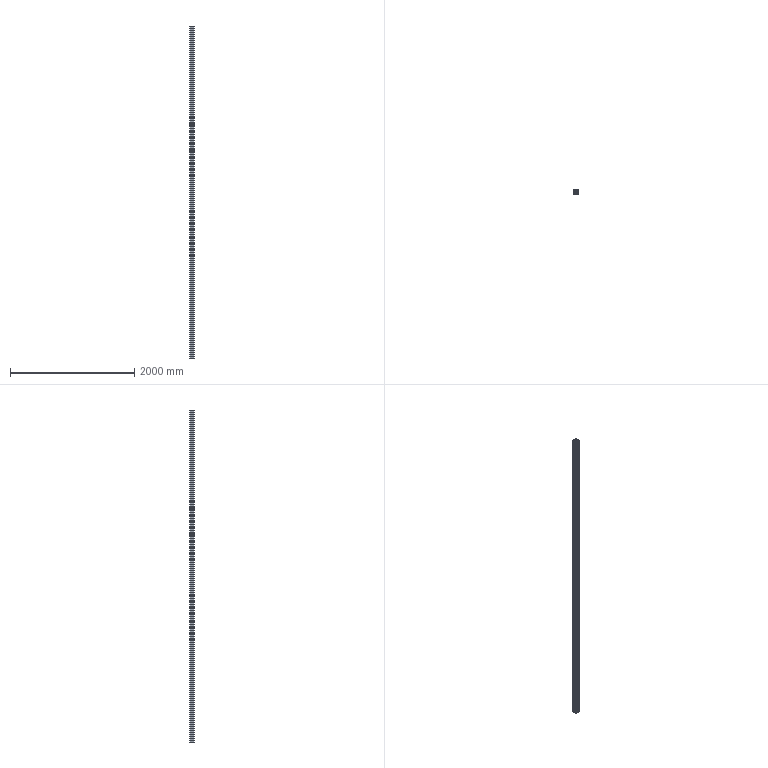Part | SolidWorks | features Extrusion 1 | 1 solid | 307 faces | box 80 x 80 x 5338 mm | volume 9294002 mm3 | plane 194 | cylinder 113 | commonest cylinder face diameters 2 x52 0.4 x16 0.6 x16 4 x9 5 x8 6.8 x8